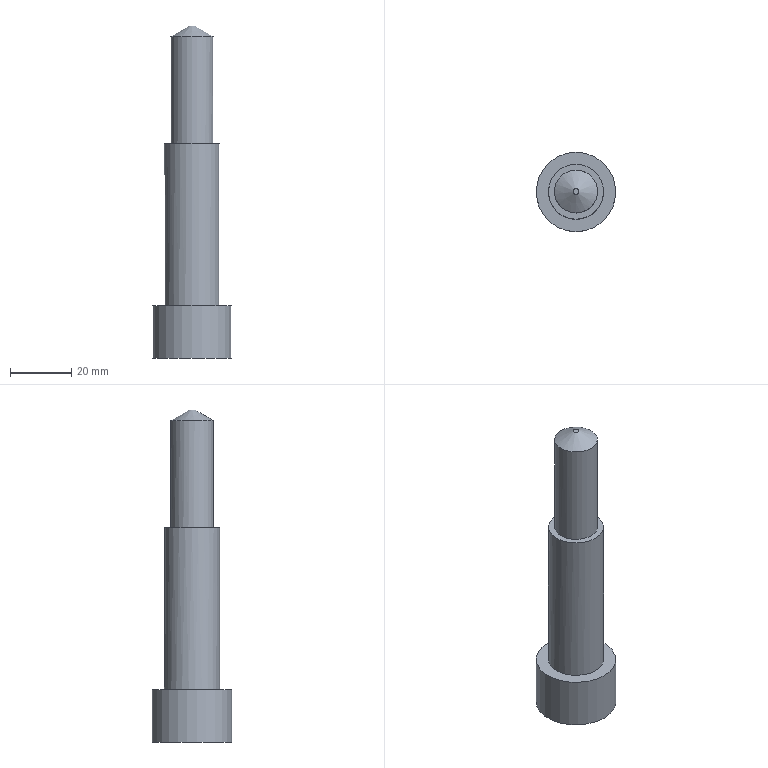Part | STEP file | solid 233 | 1 solid | 8 faces | box 26 x 26 x 108.5 mm | volume 28107 mm3 | plane 4 | cylinder 3 | cone 1 | commonest cylinder face diameters 14 x1 18 x1 26 x1